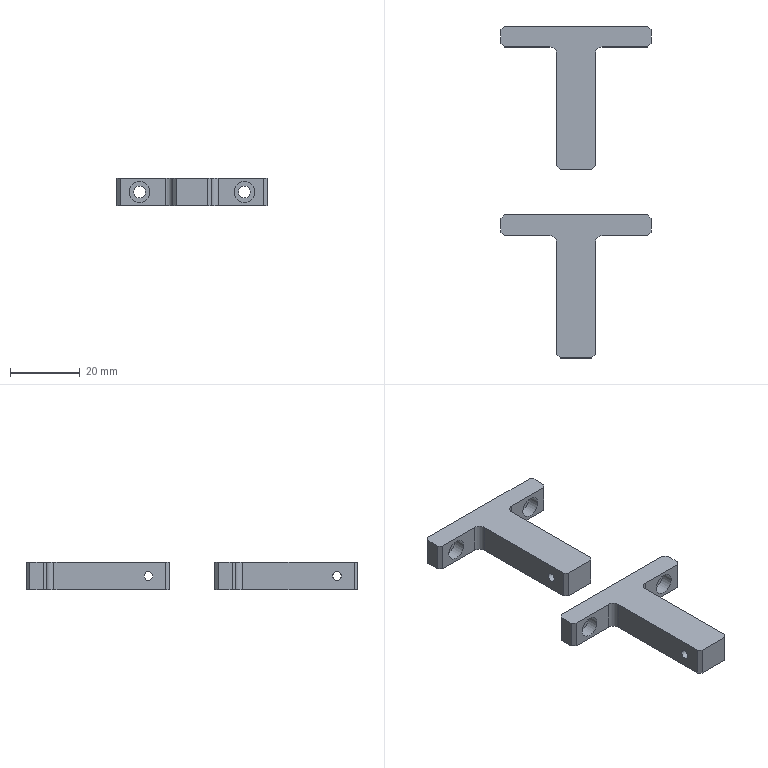Part | 2 solids | 50 faces | box 43 x 95 x 8 mm | volume 9684 mm3 | plane 36 | cylinder 14 | commonest cylinder face diameters 3.4 x4 4 x4 6 x4 2.459 x2
STEP:
#1=CARTESIAN_POINT('',(4.5,33.5,0.));
#2=VERTEX_POINT('',#1);
#3=CARTESIAN_POINT('',(-4.5,33.5,0.));
#4=VERTEX_POINT('',#3);
#5=CARTESIAN_POINT('',(21.5,33.5,0.));
#6=DIRECTION('',(-1.,0.,0.));
#7=VECTOR('',#6,1000.);
#8=LINE('',#5,#7);
#9=EDGE_CURVE('',#2,#4,#8,.T.);
#10=ORIENTED_EDGE('',*,*,#9,.T.);
#11=CARTESIAN_POINT('',(-4.5,33.5,-8.));
#12=VERTEX_POINT('',#11);
#13=CARTESIAN_POINT('',(-4.5,33.5,-8.));
#14=DIRECTION('',(0.,0.,-1.));
#15=VECTOR('',#14,1000.);
#16=LINE('',#13,#15);
#17=EDGE_CURVE('',#4,#12,#16,.T.);
#18=ORIENTED_EDGE('',*,*,#17,.T.);
#19=CARTESIAN_POINT('',(4.5,33.5,-8.));
#20=VERTEX_POINT('',#19);
#21=CARTESIAN_POINT('',(21.5,33.5,-8.));
#22=DIRECTION('',(-1.,0.,0.));
#23=VECTOR('',#22,1000.);
#24=LINE('',#21,#23);
#25=EDGE_CURVE('',#20,#12,#24,.T.);
#26=ORIENTED_EDGE('',*,*,#25,.F.);
#27=CARTESIAN_POINT('',(4.5,33.5,-8.));
#28=DIRECTION('',(0.,0.,1.));
#29=VECTOR('',#28,1000.);
#30=LINE('',#27,#29);
#31=EDGE_CURVE('',#20,#2,#30,.T.);
#32=ORIENTED_EDGE('',*,*,#31,.T.);
#33=EDGE_LOOP('',(#10,#18,#26,#32));
#34=FACE_BOUND('',#33,.T.);
#35=CARTESIAN_POINT('',(21.5,33.5,-8.));
#36=DIRECTION('',(0.,1.,0.));
#37=DIRECTION('',(0.,0.,-1.));
#38=AXIS2_PLACEMENT_3D('',#35,#36,#37);
#39=PLANE('',#38);
#40=ADVANCED_FACE('',(#34),#39,.F.);
#41=ORIENTED_EDGE('',*,*,#25,.T.);
#42=CARTESIAN_POINT('',(-5.5,34.5,-8.));
#43=VERTEX_POINT('',#42);
#44=CARTESIAN_POINT('',(-12.5,41.5,-8.));
#45=DIRECTION('',(-0.7071,0.7071,0.));
#46=VECTOR('',#45,1000.);
#47=LINE('',#44,#46);
#48=EDGE_CURVE('',#12,#43,#47,.T.);
#49=ORIENTED_EDGE('',*,*,#48,.T.);
#50=CARTESIAN_POINT('',(-5.5,66.5,-8.));
#51=VERTEX_POINT('',#50);
#52=CARTESIAN_POINT('',(-5.5,54.,-8.));
#53=DIRECTION('',(0.,1.,0.));
#54=VECTOR('',#53,1000.);
#55=LINE('',#52,#54);
#56=EDGE_CURVE('',#43,#51,#55,.T.);
#57=ORIENTED_EDGE('',*,*,#56,.T.);
#58=CARTESIAN_POINT('',(-7.5,68.5,-8.));
#59=VERTEX_POINT('',#58);
#60=CARTESIAN_POINT('',(-7.5,66.5,-8.));
#61=DIRECTION('',(0.,0.,1.));
#62=DIRECTION('',(-1.,0.,0.));
#63=AXIS2_PLACEMENT_3D('',#60,#61,#62);
#64=CIRCLE('',#63,2.);
#65=EDGE_CURVE('',#51,#59,#64,.T.);
#66=ORIENTED_EDGE('',*,*,#65,.T.);
#67=CARTESIAN_POINT('',(-20.5,68.5,-8.));
#68=VERTEX_POINT('',#67);
#69=CARTESIAN_POINT('',(0.,68.5,-8.));
#70=DIRECTION('',(-1.,0.,0.));
#71=VECTOR('',#70,1000.);
#72=LINE('',#69,#71);
#73=EDGE_CURVE('',#59,#68,#72,.T.);
#74=ORIENTED_EDGE('',*,*,#73,.T.);
#75=CARTESIAN_POINT('',(-21.5,69.5,-8.));
#76=VERTEX_POINT('',#75);
#77=CARTESIAN_POINT('',(-3.,51.,-8.));
#78=DIRECTION('',(-0.7071,0.7071,0.));
#79=VECTOR('',#78,1000.);
#80=LINE('',#77,#79);
#81=EDGE_CURVE('',#68,#76,#80,.T.);
#82=ORIENTED_EDGE('',*,*,#81,.T.);
#83=CARTESIAN_POINT('',(-21.5,73.5,-8.));
#84=VERTEX_POINT('',#83);
#85=CARTESIAN_POINT('',(-21.5,33.5,-8.));
#86=DIRECTION('',(0.,1.,0.));
#87=VECTOR('',#86,1000.);
#88=LINE('',#85,#87);
#89=EDGE_CURVE('',#76,#84,#88,.T.);
#90=ORIENTED_EDGE('',*,*,#89,.T.);
#91=CARTESIAN_POINT('',(-20.5,74.5,-8.));
#92=VERTEX_POINT('',#91);
#93=CARTESIAN_POINT('',(-20.5,74.5,-8.));
#94=DIRECTION('',(0.7071,0.7071,0.));
#95=VECTOR('',#94,1000.);
#96=LINE('',#93,#95);
#97=EDGE_CURVE('',#84,#92,#96,.T.);
#98=ORIENTED_EDGE('',*,*,#97,.T.);
#99=CARTESIAN_POINT('',(20.5,74.5,-8.));
#100=VERTEX_POINT('',#99);
#101=CARTESIAN_POINT('',(-21.5,74.5,-8.));
#102=DIRECTION('',(1.,0.,0.));
#103=VECTOR('',#102,1000.);
#104=LINE('',#101,#103);
#105=EDGE_CURVE('',#92,#100,#104,.T.);
#106=ORIENTED_EDGE('',*,*,#105,.T.);
#107=CARTESIAN_POINT('',(21.5,73.5,-8.));
#108=VERTEX_POINT('',#107);
#109=CARTESIAN_POINT('',(20.5,74.5,-8.));
#110=DIRECTION('',(0.7071,-0.7071,0.));
#111=VECTOR('',#110,1000.);
#112=LINE('',#109,#111);
#113=EDGE_CURVE('',#100,#108,#112,.T.);
#114=ORIENTED_EDGE('',*,*,#113,.T.);
#115=CARTESIAN_POINT('',(21.5,69.5,-8.));
#116=VERTEX_POINT('',#115);
#117=CARTESIAN_POINT('',(21.5,74.5,-8.));
#118=DIRECTION('',(0.,-1.,0.));
#119=VECTOR('',#118,1000.);
#120=LINE('',#117,#119);
#121=EDGE_CURVE('',#108,#116,#120,.T.);
#122=ORIENTED_EDGE('',*,*,#121,.T.);
#123=CARTESIAN_POINT('',(20.5,68.5,-8.));
#124=VERTEX_POINT('',#123);
#125=CARTESIAN_POINT('',(3.,51.,-8.));
#126=DIRECTION('',(-0.7071,-0.7071,0.));
#127=VECTOR('',#126,1000.);
#128=LINE('',#125,#127);
#129=EDGE_CURVE('',#116,#124,#128,.T.);
#130=ORIENTED_EDGE('',*,*,#129,.T.);
#131=CARTESIAN_POINT('',(7.5,68.5,-8.));
#132=VERTEX_POINT('',#131);
#133=CARTESIAN_POINT('',(0.,68.5,-8.));
#134=DIRECTION('',(1.,0.,0.));
#135=VECTOR('',#134,1000.);
#136=LINE('',#133,#135);
#137=EDGE_CURVE('',#132,#124,#136,.T.);
#138=ORIENTED_EDGE('',*,*,#137,.F.);
#139=CARTESIAN_POINT('',(5.5,66.5,-8.));
#140=VERTEX_POINT('',#139);
#141=CARTESIAN_POINT('',(7.5,66.5,-8.));
#142=DIRECTION('',(0.,0.,1.));
#143=DIRECTION('',(-1.,0.,0.));
#144=AXIS2_PLACEMENT_3D('',#141,#142,#143);
#145=CIRCLE('',#144,2.);
#146=EDGE_CURVE('',#132,#140,#145,.T.);
#147=ORIENTED_EDGE('',*,*,#146,.T.);
#148=CARTESIAN_POINT('',(5.5,34.5,-8.));
#149=VERTEX_POINT('',#148);
#150=CARTESIAN_POINT('',(5.5,54.,-8.));
#151=DIRECTION('',(0.,1.,0.));
#152=VECTOR('',#151,1000.);
#153=LINE('',#150,#152);
#154=EDGE_CURVE('',#149,#140,#153,.T.);
#155=ORIENTED_EDGE('',*,*,#154,.F.);
#156=CARTESIAN_POINT('',(12.5,41.5,-8.));
#157=DIRECTION('',(-0.7071,-0.7071,0.));
#158=VECTOR('',#157,1000.);
#159=LINE('',#156,#158);
#160=EDGE_CURVE('',#149,#20,#159,.T.);
#161=ORIENTED_EDGE('',*,*,#160,.T.);
#162=EDGE_LOOP('',(#41,#49,#57,#66,#74,#82,#90,#98,#106,#114,#122,#130,#138,#147,#155,#161));
#163=FACE_BOUND('',#162,.T.);
#164=CARTESIAN_POINT('',(0.,54.,-8.));
#165=DIRECTION('',(0.,0.,-1.));
#166=DIRECTION('',(1.,0.,0.));
#167=AXIS2_PLACEMENT_3D('',#164,#165,#166);
#168=PLANE('',#167);
#169=ADVANCED_FACE('',(#163),#168,.T.);
#170=ORIENTED_EDGE('',*,*,#121,.F.);
#171=CARTESIAN_POINT('',(21.5,73.5,0.));
#172=VERTEX_POINT('',#171);
#173=CARTESIAN_POINT('',(21.5,73.5,-8.));
#174=DIRECTION('',(0.,0.,1.));
#175=VECTOR('',#174,1000.);
#176=LINE('',#173,#175);
#177=EDGE_CURVE('',#108,#172,#176,.T.);
#178=ORIENTED_EDGE('',*,*,#177,.T.);
#179=CARTESIAN_POINT('',(21.5,69.5,0.));
#180=VERTEX_POINT('',#179);
#181=CARTESIAN_POINT('',(21.5,74.5,0.));
#182=DIRECTION('',(0.,-1.,0.));
#183=VECTOR('',#182,1000.);
#184=LINE('',#181,#183);
#185=EDGE_CURVE('',#172,#180,#184,.T.);
#186=ORIENTED_EDGE('',*,*,#185,.T.);
#187=CARTESIAN_POINT('',(21.5,69.5,-8.));
#188=DIRECTION('',(0.,0.,-1.));
#189=VECTOR('',#188,1000.);
#190=LINE('',#187,#189);
#191=EDGE_CURVE('',#180,#116,#190,.T.);
#192=ORIENTED_EDGE('',*,*,#191,.T.);
#193=EDGE_LOOP('',(#170,#178,#186,#192));
#194=FACE_BOUND('',#193,.T.);
#195=CARTESIAN_POINT('',(21.5,74.5,-8.));
#196=DIRECTION('',(-1.,0.,0.));
#197=DIRECTION('',(0.,0.,-1.));
#198=AXIS2_PLACEMENT_3D('',#195,#196,#197);
#199=PLANE('',#198);
#200=ADVANCED_FACE('',(#194),#199,.F.);
#201=CARTESIAN_POINT('',(-5.5,66.5,0.));
#202=VERTEX_POINT('',#201);
#203=CARTESIAN_POINT('',(-5.5,34.5,0.));
#204=VERTEX_POINT('',#203);
#205=CARTESIAN_POINT('',(-5.5,68.5,0.));
#206=DIRECTION('',(0.,-1.,0.));
#207=VECTOR('',#206,1000.);
#208=LINE('',#205,#207);
#209=EDGE_CURVE('',#202,#204,#208,.T.);
#210=ORIENTED_EDGE('',*,*,#209,.T.);
#211=CARTESIAN_POINT('',(-5.5,34.5,0.));
#212=DIRECTION('',(0.7071,-0.7071,0.));
#213=VECTOR('',#212,1000.);
#214=LINE('',#211,#213);
#215=EDGE_CURVE('',#204,#4,#214,.T.);
#216=ORIENTED_EDGE('',*,*,#215,.T.);
#217=ORIENTED_EDGE('',*,*,#9,.F.);
#218=CARTESIAN_POINT('',(5.5,34.5,0.));
#219=VERTEX_POINT('',#218);
#220=CARTESIAN_POINT('',(4.5,33.5,0.));
#221=DIRECTION('',(0.7071,0.7071,0.));
#222=VECTOR('',#221,1000.);
#223=LINE('',#220,#222);
#224=EDGE_CURVE('',#2,#219,#223,.T.);
#225=ORIENTED_EDGE('',*,*,#224,.T.);
#226=CARTESIAN_POINT('',(5.5,66.5,0.));
#227=VERTEX_POINT('',#226);
#228=CARTESIAN_POINT('',(5.5,68.5,0.));
#229=DIRECTION('',(0.,-1.,0.));
#230=VECTOR('',#229,1000.);
#231=LINE('',#228,#230);
#232=EDGE_CURVE('',#227,#219,#231,.T.);
#233=ORIENTED_EDGE('',*,*,#232,.F.);
#234=CARTESIAN_POINT('',(7.5,68.5,0.));
#235=VERTEX_POINT('',#234);
#236=CARTESIAN_POINT('',(7.5,66.5,0.));
#237=DIRECTION('',(0.,0.,-1.));
#238=DIRECTION('',(-1.,0.,0.));
#239=AXIS2_PLACEMENT_3D('',#236,#237,#238);
#240=CIRCLE('',#239,2.);
#241=EDGE_CURVE('',#227,#235,#240,.T.);
#242=ORIENTED_EDGE('',*,*,#241,.T.);
#243=CARTESIAN_POINT('',(20.5,68.5,0.));
#244=VERTEX_POINT('',#243);
#245=CARTESIAN_POINT('',(21.5,68.5,0.));
#246=DIRECTION('',(-1.,0.,0.));
#247=VECTOR('',#246,1000.);
#248=LINE('',#245,#247);
#249=EDGE_CURVE('',#244,#235,#248,.T.);
#250=ORIENTED_EDGE('',*,*,#249,.F.);
#251=CARTESIAN_POINT('',(20.5,68.5,0.));
#252=DIRECTION('',(0.7071,0.7071,0.));
#253=VECTOR('',#252,1000.);
#254=LINE('',#251,#253);
#255=EDGE_CURVE('',#244,#180,#254,.T.);
#256=ORIENTED_EDGE('',*,*,#255,.T.);
#257=ORIENTED_EDGE('',*,*,#185,.F.);
#258=CARTESIAN_POINT('',(20.5,74.5,0.));
#259=VERTEX_POINT('',#258);
#260=CARTESIAN_POINT('',(21.5,73.5,0.));
#261=DIRECTION('',(-0.7071,0.7071,0.));
#262=VECTOR('',#261,1000.);
#263=LINE('',#260,#262);
#264=EDGE_CURVE('',#172,#259,#263,.T.);
#265=ORIENTED_EDGE('',*,*,#264,.T.);
#266=CARTESIAN_POINT('',(-20.5,74.5,0.));
#267=VERTEX_POINT('',#266);
#268=CARTESIAN_POINT('',(-21.5,74.5,0.));
#269=DIRECTION('',(1.,0.,0.));
#270=VECTOR('',#269,1000.);
#271=LINE('',#268,#270);
#272=EDGE_CURVE('',#267,#259,#271,.T.);
#273=ORIENTED_EDGE('',*,*,#272,.F.);
#274=CARTESIAN_POINT('',(-21.5,73.5,0.));
#275=VERTEX_POINT('',#274);
#276=CARTESIAN_POINT('',(-20.5,74.5,0.));
#277=DIRECTION('',(-0.7071,-0.7071,0.));
#278=VECTOR('',#277,1000.);
#279=LINE('',#276,#278);
#280=EDGE_CURVE('',#267,#275,#279,.T.);
#281=ORIENTED_EDGE('',*,*,#280,.T.);
#282=CARTESIAN_POINT('',(-21.5,69.5,0.));
#283=VERTEX_POINT('',#282);
#284=CARTESIAN_POINT('',(-21.5,33.5,0.));
#285=DIRECTION('',(0.,1.,0.));
#286=VECTOR('',#285,1000.);
#287=LINE('',#284,#286);
#288=EDGE_CURVE('',#283,#275,#287,.T.);
#289=ORIENTED_EDGE('',*,*,#288,.F.);
#290=CARTESIAN_POINT('',(-20.5,68.5,0.));
#291=VERTEX_POINT('',#290);
#292=CARTESIAN_POINT('',(-21.5,69.5,0.));
#293=DIRECTION('',(0.7071,-0.7071,0.));
#294=VECTOR('',#293,1000.);
#295=LINE('',#292,#294);
#296=EDGE_CURVE('',#283,#291,#295,.T.);
#297=ORIENTED_EDGE('',*,*,#296,.T.);
#298=CARTESIAN_POINT('',(-7.5,68.5,0.));
#299=VERTEX_POINT('',#298);
#300=CARTESIAN_POINT('',(-21.5,68.5,0.));
#301=DIRECTION('',(1.,0.,0.));
#302=VECTOR('',#301,1000.);
#303=LINE('',#300,#302);
#304=EDGE_CURVE('',#291,#299,#303,.T.);
#305=ORIENTED_EDGE('',*,*,#304,.T.);
#306=CARTESIAN_POINT('',(-7.5,66.5,0.));
#307=DIRECTION('',(0.,0.,-1.));
#308=DIRECTION('',(-1.,0.,0.));
#309=AXIS2_PLACEMENT_3D('',#306,#307,#308);
#310=CIRCLE('',#309,2.);
#311=EDGE_CURVE('',#299,#202,#310,.T.);
#312=ORIENTED_EDGE('',*,*,#311,.T.);
#313=EDGE_LOOP('',(#210,#216,#217,#225,#233,#242,#250,#256,#257,#265,#273,#281,#289,#297,#305,#312));
#314=FACE_BOUND('',#313,.T.);
#315=CARTESIAN_POINT('',(0.,54.,0.));
#316=DIRECTION('',(0.,0.,-1.));
#317=DIRECTION('',(1.,0.,0.));
#318=AXIS2_PLACEMENT_3D('',#315,#316,#317);
#319=PLANE('',#318);
#320=ADVANCED_FACE('',(#314),#319,.F.);
#321=ORIENTED_EDGE('',*,*,#89,.F.);
#322=CARTESIAN_POINT('',(-21.5,69.5,0.));
#323=DIRECTION('',(0.,0.,1.));
#324=VECTOR('',#323,1000.);
#325=LINE('',#322,#324);
#326=EDGE_CURVE('',#76,#283,#325,.T.);
#327=ORIENTED_EDGE('',*,*,#326,.T.);
#328=ORIENTED_EDGE('',*,*,#288,.T.);
#329=CARTESIAN_POINT('',(-21.5,73.5,-8.));
#330=DIRECTION('',(0.,0.,-1.));
#331=VECTOR('',#330,1000.);
#332=LINE('',#329,#331);
#333=EDGE_CURVE('',#275,#84,#332,.T.);
#334=ORIENTED_EDGE('',*,*,#333,.T.);
#335=EDGE_LOOP('',(#321,#327,#328,#334));
#336=FACE_BOUND('',#335,.T.);
#337=CARTESIAN_POINT('',(-21.5,33.5,-8.));
#338=DIRECTION('',(1.,0.,0.));
#339=DIRECTION('',(0.,0.,1.));
#340=AXIS2_PLACEMENT_3D('',#337,#338,#339);
#341=PLANE('',#340);
#342=ADVANCED_FACE('',(#336),#341,.F.);
#343=CARTESIAN_POINT('',(15.,74.5,-5.7));
#344=VERTEX_POINT('',#343);
#345=CARTESIAN_POINT('',(15.,74.5,-4.));
#346=DIRECTION('',(0.,-1.,0.));
#347=DIRECTION('',(0.,0.,-1.));
#348=AXIS2_PLACEMENT_3D('',#345,#346,#347);
#349=CIRCLE('',#348,1.7);
#350=EDGE_CURVE('',#344,#344,#349,.T.);
#351=ORIENTED_EDGE('',*,*,#350,.T.);
#352=EDGE_LOOP('',(#351));
#353=FACE_BOUND('',#352,.T.);
#354=CARTESIAN_POINT('',(-15.,74.5,-5.7));
#355=VERTEX_POINT('',#354);
#356=CARTESIAN_POINT('',(-15.,74.5,-4.));
#357=DIRECTION('',(0.,-1.,0.));
#358=DIRECTION('',(0.,0.,-1.));
#359=AXIS2_PLACEMENT_3D('',#356,#357,#358);
#360=CIRCLE('',#359,1.7);
#361=EDGE_CURVE('',#355,#355,#360,.T.);
#362=ORIENTED_EDGE('',*,*,#361,.T.);
#363=EDGE_LOOP('',(#362));
#364=FACE_BOUND('',#363,.T.);
#365=ORIENTED_EDGE('',*,*,#105,.F.);
#366=CARTESIAN_POINT('',(-20.5,74.5,-8.));
#367=DIRECTION('',(0.,0.,1.));
#368=VECTOR('',#367,1000.);
#369=LINE('',#366,#368);
#370=EDGE_CURVE('',#92,#267,#369,.T.);
#371=ORIENTED_EDGE('',*,*,#370,.T.);
#372=ORIENTED_EDGE('',*,*,#272,.T.);
#373=CARTESIAN_POINT('',(20.5,74.5,-8.));
#374=DIRECTION('',(0.,0.,-1.));
#375=VECTOR('',#374,1000.);
#376=LINE('',#373,#375);
#377=EDGE_CURVE('',#259,#100,#376,.T.);
#378=ORIENTED_EDGE('',*,*,#377,.T.);
#379=EDGE_LOOP('',(#365,#371,#372,#378));
#380=FACE_BOUND('',#379,.T.);
#381=CARTESIAN_POINT('',(-21.5,74.5,-8.));
#382=DIRECTION('',(0.,-1.,0.));
#383=DIRECTION('',(0.,0.,1.));
#384=AXIS2_PLACEMENT_3D('',#381,#382,#383);
#385=PLANE('',#384);
#386=ADVANCED_FACE('',(#353,#364,#380),#385,.F.);
#387=CARTESIAN_POINT('',(15.,68.5,-7.));
#388=VERTEX_POINT('',#387);
#389=CARTESIAN_POINT('',(15.,68.5,-4.));
#390=DIRECTION('',(0.,1.,0.));
#391=DIRECTION('',(0.,0.,-1.));
#392=AXIS2_PLACEMENT_3D('',#389,#390,#391);
#393=CIRCLE('',#392,3.);
#394=EDGE_CURVE('',#388,#388,#393,.T.);
#395=ORIENTED_EDGE('',*,*,#394,.T.);
#396=EDGE_LOOP('',(#395));
#397=FACE_BOUND('',#396,.T.);
#398=ORIENTED_EDGE('',*,*,#249,.T.);
#399=CARTESIAN_POINT('',(7.5,68.5,-8.));
#400=DIRECTION('',(0.,0.,-1.));
#401=VECTOR('',#400,1000.);
#402=LINE('',#399,#401);
#403=EDGE_CURVE('',#235,#132,#402,.T.);
#404=ORIENTED_EDGE('',*,*,#403,.T.);
#405=ORIENTED_EDGE('',*,*,#137,.T.);
#406=CARTESIAN_POINT('',(20.5,68.5,-103.5));
#407=DIRECTION('',(0.,0.,1.));
#408=VECTOR('',#407,1000.);
#409=LINE('',#406,#408);
#410=EDGE_CURVE('',#124,#244,#409,.T.);
#411=ORIENTED_EDGE('',*,*,#410,.T.);
#412=EDGE_LOOP('',(#398,#404,#405,#411));
#413=FACE_BOUND('',#412,.T.);
#414=CARTESIAN_POINT('',(21.5,68.5,-103.5));
#415=DIRECTION('',(0.,1.,0.));
#416=DIRECTION('',(0.,0.,-1.));
#417=AXIS2_PLACEMENT_3D('',#414,#415,#416);
#418=PLANE('',#417);
#419=ADVANCED_FACE('',(#397,#413),#418,.F.);
#420=CARTESIAN_POINT('',(5.5,40.73,-4.));
#421=VERTEX_POINT('',#420);
#422=CARTESIAN_POINT('',(5.5,39.5,-4.));
#423=DIRECTION('',(-1.,0.,0.));
#424=DIRECTION('',(0.,1.,0.));
#425=AXIS2_PLACEMENT_3D('',#422,#423,#424);
#426=CIRCLE('',#425,1.23);
#427=EDGE_CURVE('',#421,#421,#426,.T.);
#428=ORIENTED_EDGE('',*,*,#427,.T.);
#429=EDGE_LOOP('',(#428));
#430=FACE_BOUND('',#429,.T.);
#431=ORIENTED_EDGE('',*,*,#154,.T.);
#432=CARTESIAN_POINT('',(5.5,66.5,0.));
#433=DIRECTION('',(0.,0.,1.));
#434=VECTOR('',#433,1000.);
#435=LINE('',#432,#434);
#436=EDGE_CURVE('',#140,#227,#435,.T.);
#437=ORIENTED_EDGE('',*,*,#436,.T.);
#438=ORIENTED_EDGE('',*,*,#232,.T.);
#439=CARTESIAN_POINT('',(5.5,34.5,-103.5));
#440=DIRECTION('',(0.,0.,-1.));
#441=VECTOR('',#440,1000.);
#442=LINE('',#439,#441);
#443=EDGE_CURVE('',#219,#149,#442,.T.);
#444=ORIENTED_EDGE('',*,*,#443,.T.);
#445=EDGE_LOOP('',(#431,#437,#438,#444));
#446=FACE_BOUND('',#445,.T.);
#447=CARTESIAN_POINT('',(5.5,68.5,-103.5));
#448=DIRECTION('',(-1.,0.,0.));
#449=DIRECTION('',(0.,1.,0.));
#450=AXIS2_PLACEMENT_3D('',#447,#448,#449);
#451=PLANE('',#450);
#452=ADVANCED_FACE('',(#430,#446),#451,.F.);
#453=CARTESIAN_POINT('',(-15.,68.5,-7.));
#454=VERTEX_POINT('',#453);
#455=CARTESIAN_POINT('',(-15.,68.5,-4.));
#456=DIRECTION('',(0.,1.,0.));
#457=DIRECTION('',(0.,0.,-1.));
#458=AXIS2_PLACEMENT_3D('',#455,#456,#457);
#459=CIRCLE('',#458,3.);
#460=EDGE_CURVE('',#454,#454,#459,.T.);
#461=ORIENTED_EDGE('',*,*,#460,.T.);
#462=EDGE_LOOP('',(#461));
#463=FACE_BOUND('',#462,.T.);
#464=ORIENTED_EDGE('',*,*,#304,.F.);
#465=CARTESIAN_POINT('',(-20.5,68.5,-8.));
#466=DIRECTION('',(0.,0.,-1.));
#467=VECTOR('',#466,1000.);
#468=LINE('',#465,#467);
#469=EDGE_CURVE('',#291,#68,#468,.T.);
#470=ORIENTED_EDGE('',*,*,#469,.T.);
#471=ORIENTED_EDGE('',*,*,#73,.F.);
#472=CARTESIAN_POINT('',(-7.5,68.5,0.));
#473=DIRECTION('',(0.,0.,1.));
#474=VECTOR('',#473,1000.);
#475=LINE('',#472,#474);
#476=EDGE_CURVE('',#59,#299,#475,.T.);
#477=ORIENTED_EDGE('',*,*,#476,.T.);
#478=EDGE_LOOP('',(#464,#470,#471,#477));
#479=FACE_BOUND('',#478,.T.);
#480=CARTESIAN_POINT('',(-21.5,68.5,-103.5));
#481=DIRECTION('',(0.,-1.,0.));
#482=DIRECTION('',(-1.,0.,0.));
#483=AXIS2_PLACEMENT_3D('',#480,#481,#482);
#484=PLANE('',#483);
#485=ADVANCED_FACE('',(#463,#479),#484,.T.);
#486=CARTESIAN_POINT('',(-5.5,38.27,-4.));
#487=VERTEX_POINT('',#486);
#488=CARTESIAN_POINT('',(-5.5,39.5,-4.));
#489=DIRECTION('',(-1.,0.,0.));
#490=DIRECTION('',(0.,-1.,0.));
#491=AXIS2_PLACEMENT_3D('',#488,#489,#490);
#492=CIRCLE('',#491,1.23);
#493=EDGE_CURVE('',#487,#487,#492,.T.);
#494=ORIENTED_EDGE('',*,*,#493,.F.);
#495=EDGE_LOOP('',(#494));
#496=FACE_BOUND('',#495,.T.);
#497=ORIENTED_EDGE('',*,*,#56,.F.);
#498=CARTESIAN_POINT('',(-5.5,34.5,0.));
#499=DIRECTION('',(0.,0.,1.));
#500=VECTOR('',#499,1000.);
#501=LINE('',#498,#500);
#502=EDGE_CURVE('',#43,#204,#501,.T.);
#503=ORIENTED_EDGE('',*,*,#502,.T.);
#504=ORIENTED_EDGE('',*,*,#209,.F.);
#505=CARTESIAN_POINT('',(-5.5,66.5,-8.));
#506=DIRECTION('',(0.,0.,-1.));
#507=VECTOR('',#506,1000.);
#508=LINE('',#505,#507);
#509=EDGE_CURVE('',#202,#51,#508,.T.);
#510=ORIENTED_EDGE('',*,*,#509,.T.);
#511=EDGE_LOOP('',(#497,#503,#504,#510));
#512=FACE_BOUND('',#511,.T.);
#513=CARTESIAN_POINT('',(-5.5,68.5,-103.5));
#514=DIRECTION('',(-1.,0.,0.));
#515=DIRECTION('',(0.,1.,0.));
#516=AXIS2_PLACEMENT_3D('',#513,#514,#515);
#517=PLANE('',#516);
#518=ADVANCED_FACE('',(#496,#512),#517,.T.);
#519=ORIENTED_EDGE('',*,*,#160,.F.);
#520=ORIENTED_EDGE('',*,*,#443,.F.);
#521=ORIENTED_EDGE('',*,*,#224,.F.);
#522=ORIENTED_EDGE('',*,*,#31,.F.);
#523=EDGE_LOOP('',(#519,#520,#521,#522));
#524=FACE_BOUND('',#523,.T.);
#525=CARTESIAN_POINT('',(4.5,33.5,-8.));
#526=DIRECTION('',(-0.7071,0.7071,0.));
#527=DIRECTION('',(0.,0.,-1.));
#528=AXIS2_PLACEMENT_3D('',#525,#526,#527);
#529=PLANE('',#528);
#530=ADVANCED_FACE('',(#524),#529,.F.);
#531=ORIENTED_EDGE('',*,*,#97,.F.);
#532=ORIENTED_EDGE('',*,*,#333,.F.);
#533=ORIENTED_EDGE('',*,*,#280,.F.);
#534=ORIENTED_EDGE('',*,*,#370,.F.);
#535=EDGE_LOOP('',(#531,#532,#533,#534));
#536=FACE_BOUND('',#535,.T.);
#537=CARTESIAN_POINT('',(-20.5,74.5,-8.));
#538=DIRECTION('',(0.7071,-0.7071,0.));
#539=DIRECTION('',(0.,0.,-1.));
#540=AXIS2_PLACEMENT_3D('',#537,#538,#539);
#541=PLANE('',#540);
#542=ADVANCED_FACE('',(#536),#541,.F.);
#543=ORIENTED_EDGE('',*,*,#113,.F.);
#544=ORIENTED_EDGE('',*,*,#377,.F.);
#545=ORIENTED_EDGE('',*,*,#264,.F.);
#546=ORIENTED_EDGE('',*,*,#177,.F.);
#547=EDGE_LOOP('',(#543,#544,#545,#546));
#548=FACE_BOUND('',#547,.T.);
#549=CARTESIAN_POINT('',(21.5,73.5,-8.));
#550=DIRECTION('',(-0.7071,-0.7071,0.));
#551=DIRECTION('',(0.,0.,-1.));
#552=AXIS2_PLACEMENT_3D('',#549,#550,#551);
#553=PLANE('',#552);
#554=ADVANCED_FACE('',(#548),#553,.F.);
#555=ORIENTED_EDGE('',*,*,#129,.F.);
#556=ORIENTED_EDGE('',*,*,#191,.F.);
#557=ORIENTED_EDGE('',*,*,#255,.F.);
#558=ORIENTED_EDGE('',*,*,#410,.F.);
#559=EDGE_LOOP('',(#555,#556,#557,#558));
#560=FACE_BOUND('',#559,.T.);
#561=CARTESIAN_POINT('',(20.5,68.5,-103.5));
#562=DIRECTION('',(-0.7071,0.7071,0.));
#563=DIRECTION('',(0.,0.,-1.));
#564=AXIS2_PLACEMENT_3D('',#561,#562,#563);
#565=PLANE('',#564);
#566=ADVANCED_FACE('',(#560),#565,.F.);
#567=ORIENTED_EDGE('',*,*,#146,.F.);
#568=ORIENTED_EDGE('',*,*,#403,.F.);
#569=ORIENTED_EDGE('',*,*,#241,.F.);
#570=ORIENTED_EDGE('',*,*,#436,.F.);
#571=EDGE_LOOP('',(#567,#568,#569,#570));
#572=FACE_BOUND('',#571,.T.);
#573=CARTESIAN_POINT('',(7.5,66.5,-103.5));
#574=DIRECTION('',(0.,0.,-1.));
#575=DIRECTION('',(1.,0.,0.));
#576=AXIS2_PLACEMENT_3D('',#573,#574,#575);
#577=CYLINDRICAL_SURFACE('',#576,2.);
#578=ADVANCED_FACE('',(#572),#577,.F.);
#579=ORIENTED_EDGE('',*,*,#65,.F.);
#580=ORIENTED_EDGE('',*,*,#509,.F.);
#581=ORIENTED_EDGE('',*,*,#311,.F.);
#582=ORIENTED_EDGE('',*,*,#476,.F.);
#583=EDGE_LOOP('',(#579,#580,#581,#582));
#584=FACE_BOUND('',#583,.T.);
#585=CARTESIAN_POINT('',(-7.5,66.5,-103.5));
#586=DIRECTION('',(0.,0.,-1.));
#587=DIRECTION('',(1.,0.,0.));
#588=AXIS2_PLACEMENT_3D('',#585,#586,#587);
#589=CYLINDRICAL_SURFACE('',#588,2.);
#590=ADVANCED_FACE('',(#584),#589,.F.);
#591=CARTESIAN_POINT('',(-15.,71.9,-5.7));
#592=VERTEX_POINT('',#591);
#593=CARTESIAN_POINT('',(-15.,71.9,-4.));
#594=DIRECTION('',(0.,1.,0.));
#595=DIRECTION('',(0.,0.,-1.));
#596=AXIS2_PLACEMENT_3D('',#593,#594,#595);
#597=CIRCLE('',#596,1.7);
#598=EDGE_CURVE('',#592,#592,#597,.T.);
#599=ORIENTED_EDGE('',*,*,#598,.F.);
#600=EDGE_LOOP('',(#599));
#601=FACE_BOUND('',#600,.T.);
#602=ORIENTED_EDGE('',*,*,#361,.F.);
#603=EDGE_LOOP('',(#602));
#604=FACE_BOUND('',#603,.T.);
#605=CARTESIAN_POINT('',(-15.,71.9,-4.));
#606=DIRECTION('',(0.,1.,0.));
#607=DIRECTION('',(0.,0.,1.));
#608=AXIS2_PLACEMENT_3D('',#605,#606,#607);
#609=CYLINDRICAL_SURFACE('',#608,1.7);
#610=ADVANCED_FACE('',(#601,#604),#609,.F.);
#611=ORIENTED_EDGE('',*,*,#598,.T.);
#612=EDGE_LOOP('',(#611));
#613=FACE_BOUND('',#612,.T.);
#614=CARTESIAN_POINT('',(-15.,71.9,-7.));
#615=VERTEX_POINT('',#614);
#616=CARTESIAN_POINT('',(-15.,71.9,-4.));
#617=DIRECTION('',(0.,-1.,0.));
#618=DIRECTION('',(0.,0.,-1.));
#619=AXIS2_PLACEMENT_3D('',#616,#617,#618);
#620=CIRCLE('',#619,3.);
#621=EDGE_CURVE('',#615,#615,#620,.T.);
#622=ORIENTED_EDGE('',*,*,#621,.T.);
#623=EDGE_LOOP('',(#622));
#624=FACE_BOUND('',#623,.T.);
#625=CARTESIAN_POINT('',(-15.,71.9,-4.));
#626=DIRECTION('',(0.,1.,0.));
#627=DIRECTION('',(0.,0.,-1.));
#628=AXIS2_PLACEMENT_3D('',#625,#626,#627);
#629=PLANE('',#628);
#630=ADVANCED_FACE('',(#613,#624),#629,.F.);
#631=ORIENTED_EDGE('',*,*,#621,.F.);
#632=EDGE_LOOP('',(#631));
#633=FACE_BOUND('',#632,.T.);
#634=ORIENTED_EDGE('',*,*,#460,.F.);
#635=EDGE_LOOP('',(#634));
#636=FACE_BOUND('',#635,.T.);
#637=CARTESIAN_POINT('',(-15.,68.5,-4.));
#638=DIRECTION('',(0.,1.,0.));
#639=DIRECTION('',(0.,0.,1.));
#640=AXIS2_PLACEMENT_3D('',#637,#638,#639);
#641=CYLINDRICAL_SURFACE('',#640,3.);
#642=ADVANCED_FACE('',(#633,#636),#641,.F.);
#643=CARTESIAN_POINT('',(15.,71.9,-5.7));
#644=VERTEX_POINT('',#643);
#645=CARTESIAN_POINT('',(15.,71.9,-4.));
#646=DIRECTION('',(0.,1.,0.));
#647=DIRECTION('',(0.,0.,-1.));
#648=AXIS2_PLACEMENT_3D('',#645,#646,#647);
#649=CIRCLE('',#648,1.7);
#650=EDGE_CURVE('',#644,#644,#649,.T.);
#651=ORIENTED_EDGE('',*,*,#650,.F.);
#652=EDGE_LOOP('',(#651));
#653=FACE_BOUND('',#652,.T.);
#654=ORIENTED_EDGE('',*,*,#350,.F.);
#655=EDGE_LOOP('',(#654));
#656=FACE_BOUND('',#655,.T.);
#657=CARTESIAN_POINT('',(15.,71.9,-4.));
#658=DIRECTION('',(0.,1.,0.));
#659=DIRECTION('',(0.,0.,1.));
#660=AXIS2_PLACEMENT_3D('',#657,#658,#659);
#661=CYLINDRICAL_SURFACE('',#660,1.7);
#662=ADVANCED_FACE('',(#653,#656),#661,.F.);
#663=ORIENTED_EDGE('',*,*,#650,.T.);
#664=EDGE_LOOP('',(#663));
#665=FACE_BOUND('',#664,.T.);
#666=CARTESIAN_POINT('',(15.,71.9,-7.));
#667=VERTEX_POINT('',#666);
#668=CARTESIAN_POINT('',(15.,71.9,-4.));
#669=DIRECTION('',(0.,-1.,0.));
#670=DIRECTION('',(0.,0.,-1.));
#671=AXIS2_PLACEMENT_3D('',#668,#669,#670);
#672=CIRCLE('',#671,3.);
#673=EDGE_CURVE('',#667,#667,#672,.T.);
#674=ORIENTED_EDGE('',*,*,#673,.T.);
#675=EDGE_LOOP('',(#674));
#676=FACE_BOUND('',#675,.T.);
#677=CARTESIAN_POINT('',(15.,71.9,-4.));
#678=DIRECTION('',(0.,1.,0.));
#679=DIRECTION('',(0.,0.,-1.));
#680=AXIS2_PLACEMENT_3D('',#677,#678,#679);
#681=PLANE('',#680);
#682=ADVANCED_FACE('',(#665,#676),#681,.F.);
#683=ORIENTED_EDGE('',*,*,#673,.F.);
#684=EDGE_LOOP('',(#683));
#685=FACE_BOUND('',#684,.T.);
#686=ORIENTED_EDGE('',*,*,#394,.F.);
#687=EDGE_LOOP('',(#686));
#688=FACE_BOUND('',#687,.T.);
#689=CARTESIAN_POINT('',(15.,68.5,-4.));
#690=DIRECTION('',(0.,1.,0.));
#691=DIRECTION('',(0.,0.,1.));
#692=AXIS2_PLACEMENT_3D('',#689,#690,#691);
#693=CYLINDRICAL_SURFACE('',#692,3.);
#694=ADVANCED_FACE('',(#685,#688),#693,.F.);
#695=ORIENTED_EDGE('',*,*,#493,.T.);
#696=EDGE_LOOP('',(#695));
#697=FACE_BOUND('',#696,.T.);
#698=ORIENTED_EDGE('',*,*,#427,.F.);
#699=EDGE_LOOP('',(#698));
#700=FACE_BOUND('',#699,.T.);
#701=CARTESIAN_POINT('',(5.5,39.5,-4.));
#702=DIRECTION('',(-1.,0.,0.));
#703=DIRECTION('',(0.,-1.,0.));
#704=AXIS2_PLACEMENT_3D('',#701,#702,#703);
#705=CYLINDRICAL_SURFACE('',#704,1.23);
#706=ADVANCED_FACE('',(#697,#700),#705,.F.);
#707=ORIENTED_EDGE('',*,*,#81,.F.);
#708=ORIENTED_EDGE('',*,*,#469,.F.);
#709=ORIENTED_EDGE('',*,*,#296,.F.);
#710=ORIENTED_EDGE('',*,*,#326,.F.);
#711=EDGE_LOOP('',(#707,#708,#709,#710));
#712=FACE_BOUND('',#711,.T.);
#713=CARTESIAN_POINT('',(-21.5,69.5,-8.));
#714=DIRECTION('',(-0.7071,-0.7071,0.));
#715=DIRECTION('',(0.,0.,1.));
#716=AXIS2_PLACEMENT_3D('',#713,#714,#715);
#717=PLANE('',#716);
#718=ADVANCED_FACE('',(#712),#717,.T.);
#719=ORIENTED_EDGE('',*,*,#48,.F.);
#720=ORIENTED_EDGE('',*,*,#17,.F.);
#721=ORIENTED_EDGE('',*,*,#215,.F.);
#722=ORIENTED_EDGE('',*,*,#502,.F.);
#723=EDGE_LOOP('',(#719,#720,#721,#722));
#724=FACE_BOUND('',#723,.T.);
#725=CARTESIAN_POINT('',(-5.5,34.5,-103.5));
#726=DIRECTION('',(-0.7071,-0.7071,0.));
#727=DIRECTION('',(0.,0.,1.));
#728=AXIS2_PLACEMENT_3D('',#725,#726,#727);
#729=PLANE('',#728);
#730=ADVANCED_FACE('',(#724),#729,.T.);
#731=CLOSED_SHELL('',(#40,#169,#200,#320,#342,#386,#419,#452,#485,#518,#530,#542,#554,#566,#578,#590,#610,#630,#642,#662,#682,#694,#706,#718,#730));
#732=MANIFOLD_SOLID_BREP('',#731);
#733=CARTESIAN_POINT('',(4.5,-20.5,0.));
#734=VERTEX_POINT('',#733);
#735=CARTESIAN_POINT('',(-4.5,-20.5,0.));
#736=VERTEX_POINT('',#735);
#737=CARTESIAN_POINT('',(21.5,-20.5,0.));
#738=DIRECTION('',(-1.,0.,0.));
#739=VECTOR('',#738,1000.);
#740=LINE('',#737,#739);
#741=EDGE_CURVE('',#734,#736,#740,.T.);
#742=ORIENTED_EDGE('',*,*,#741,.T.);
#743=CARTESIAN_POINT('',(-4.5,-20.5,-8.));
#744=VERTEX_POINT('',#743);
#745=CARTESIAN_POINT('',(-4.5,-20.5,-8.));
#746=DIRECTION('',(0.,0.,-1.));
#747=VECTOR('',#746,1000.);
#748=LINE('',#745,#747);
#749=EDGE_CURVE('',#736,#744,#748,.T.);
#750=ORIENTED_EDGE('',*,*,#749,.T.);
#751=CARTESIAN_POINT('',(4.5,-20.5,-8.));
#752=VERTEX_POINT('',#751);
#753=CARTESIAN_POINT('',(21.5,-20.5,-8.));
#754=DIRECTION('',(-1.,0.,0.));
#755=VECTOR('',#754,1000.);
#756=LINE('',#753,#755);
#757=EDGE_CURVE('',#752,#744,#756,.T.);
#758=ORIENTED_EDGE('',*,*,#757,.F.);
#759=CARTESIAN_POINT('',(4.5,-20.5,-8.));
#760=DIRECTION('',(0.,0.,1.));
#761=VECTOR('',#760,1000.);
#762=LINE('',#759,#761);
#763=EDGE_CURVE('',#752,#734,#762,.T.);
#764=ORIENTED_EDGE('',*,*,#763,.T.);
#765=EDGE_LOOP('',(#742,#750,#758,#764));
#766=FACE_BOUND('',#765,.T.);
#767=CARTESIAN_POINT('',(21.5,-20.5,-8.));
#768=DIRECTION('',(0.,1.,0.));
#769=DIRECTION('',(0.,0.,-1.));
#770=AXIS2_PLACEMENT_3D('',#767,#768,#769);
#771=PLANE('',#770);
#772=ADVANCED_FACE('',(#766),#771,.F.);
#773=ORIENTED_EDGE('',*,*,#757,.T.);
#774=CARTESIAN_POINT('',(-5.5,-19.5,-8.));
#775=VERTEX_POINT('',#774);
#776=CARTESIAN_POINT('',(-12.5,-12.5,-8.));
#777=DIRECTION('',(-0.7071,0.7071,0.));
#778=VECTOR('',#777,1000.);
#779=LINE('',#776,#778);
#780=EDGE_CURVE('',#744,#775,#779,.T.);
#781=ORIENTED_EDGE('',*,*,#780,.T.);
#782=CARTESIAN_POINT('',(-5.5,12.5,-8.));
#783=VERTEX_POINT('',#782);
#784=CARTESIAN_POINT('',(-5.5,0.,-8.));
#785=DIRECTION('',(0.,1.,0.));
#786=VECTOR('',#785,1000.);
#787=LINE('',#784,#786);
#788=EDGE_CURVE('',#775,#783,#787,.T.);
#789=ORIENTED_EDGE('',*,*,#788,.T.);
#790=CARTESIAN_POINT('',(-7.5,14.5,-8.));
#791=VERTEX_POINT('',#790);
#792=CARTESIAN_POINT('',(-7.5,12.5,-8.));
#793=DIRECTION('',(0.,0.,1.));
#794=DIRECTION('',(-1.,0.,0.));
#795=AXIS2_PLACEMENT_3D('',#792,#793,#794);
#796=CIRCLE('',#795,2.);
#797=EDGE_CURVE('',#783,#791,#796,.T.);
#798=ORIENTED_EDGE('',*,*,#797,.T.);
#799=CARTESIAN_POINT('',(-20.5,14.5,-8.));
#800=VERTEX_POINT('',#799);
#801=CARTESIAN_POINT('',(0.,14.5,-8.));
#802=DIRECTION('',(-1.,0.,0.));
#803=VECTOR('',#802,1000.);
#804=LINE('',#801,#803);
#805=EDGE_CURVE('',#791,#800,#804,.T.);
#806=ORIENTED_EDGE('',*,*,#805,.T.);
#807=CARTESIAN_POINT('',(-21.5,15.5,-8.));
#808=VERTEX_POINT('',#807);
#809=CARTESIAN_POINT('',(-3.,-3.,-8.));
#810=DIRECTION('',(-0.7071,0.7071,0.));
#811=VECTOR('',#810,1000.);
#812=LINE('',#809,#811);
#813=EDGE_CURVE('',#800,#808,#812,.T.);
#814=ORIENTED_EDGE('',*,*,#813,.T.);
#815=CARTESIAN_POINT('',(-21.5,19.5,-8.));
#816=VERTEX_POINT('',#815);
#817=CARTESIAN_POINT('',(-21.5,-20.5,-8.));
#818=DIRECTION('',(0.,1.,0.));
#819=VECTOR('',#818,1000.);
#820=LINE('',#817,#819);
#821=EDGE_CURVE('',#808,#816,#820,.T.);
#822=ORIENTED_EDGE('',*,*,#821,.T.);
#823=CARTESIAN_POINT('',(-20.5,20.5,-8.));
#824=VERTEX_POINT('',#823);
#825=CARTESIAN_POINT('',(-20.5,20.5,-8.));
#826=DIRECTION('',(0.7071,0.7071,0.));
#827=VECTOR('',#826,1000.);
#828=LINE('',#825,#827);
#829=EDGE_CURVE('',#816,#824,#828,.T.);
#830=ORIENTED_EDGE('',*,*,#829,.T.);
#831=CARTESIAN_POINT('',(20.5,20.5,-8.));
#832=VERTEX_POINT('',#831);
#833=CARTESIAN_POINT('',(-21.5,20.5,-8.));
#834=DIRECTION('',(1.,0.,0.));
#835=VECTOR('',#834,1000.);
#836=LINE('',#833,#835);
#837=EDGE_CURVE('',#824,#832,#836,.T.);
#838=ORIENTED_EDGE('',*,*,#837,.T.);
#839=CARTESIAN_POINT('',(21.5,19.5,-8.));
#840=VERTEX_POINT('',#839);
#841=CARTESIAN_POINT('',(20.5,20.5,-8.));
#842=DIRECTION('',(0.7071,-0.7071,0.));
#843=VECTOR('',#842,1000.);
#844=LINE('',#841,#843);
#845=EDGE_CURVE('',#832,#840,#844,.T.);
#846=ORIENTED_EDGE('',*,*,#845,.T.);
#847=CARTESIAN_POINT('',(21.5,15.5,-8.));
#848=VERTEX_POINT('',#847);
#849=CARTESIAN_POINT('',(21.5,20.5,-8.));
#850=DIRECTION('',(0.,-1.,0.));
#851=VECTOR('',#850,1000.);
#852=LINE('',#849,#851);
#853=EDGE_CURVE('',#840,#848,#852,.T.);
#854=ORIENTED_EDGE('',*,*,#853,.T.);
#855=CARTESIAN_POINT('',(20.5,14.5,-8.));
#856=VERTEX_POINT('',#855);
#857=CARTESIAN_POINT('',(3.,-3.,-8.));
#858=DIRECTION('',(-0.7071,-0.7071,0.));
#859=VECTOR('',#858,1000.);
#860=LINE('',#857,#859);
#861=EDGE_CURVE('',#848,#856,#860,.T.);
#862=ORIENTED_EDGE('',*,*,#861,.T.);
#863=CARTESIAN_POINT('',(7.5,14.5,-8.));
#864=VERTEX_POINT('',#863);
#865=CARTESIAN_POINT('',(0.,14.5,-8.));
#866=DIRECTION('',(1.,0.,0.));
#867=VECTOR('',#866,1000.);
#868=LINE('',#865,#867);
#869=EDGE_CURVE('',#864,#856,#868,.T.);
#870=ORIENTED_EDGE('',*,*,#869,.F.);
#871=CARTESIAN_POINT('',(5.5,12.5,-8.));
#872=VERTEX_POINT('',#871);
#873=CARTESIAN_POINT('',(7.5,12.5,-8.));
#874=DIRECTION('',(0.,0.,1.));
#875=DIRECTION('',(-1.,0.,0.));
#876=AXIS2_PLACEMENT_3D('',#873,#874,#875);
#877=CIRCLE('',#876,2.);
#878=EDGE_CURVE('',#864,#872,#877,.T.);
#879=ORIENTED_EDGE('',*,*,#878,.T.);
#880=CARTESIAN_POINT('',(5.5,-19.5,-8.));
#881=VERTEX_POINT('',#880);
#882=CARTESIAN_POINT('',(5.5,0.,-8.));
#883=DIRECTION('',(0.,1.,0.));
#884=VECTOR('',#883,1000.);
#885=LINE('',#882,#884);
#886=EDGE_CURVE('',#881,#872,#885,.T.);
#887=ORIENTED_EDGE('',*,*,#886,.F.);
#888=CARTESIAN_POINT('',(12.5,-12.5,-8.));
#889=DIRECTION('',(-0.7071,-0.7071,0.));
#890=VECTOR('',#889,1000.);
#891=LINE('',#888,#890);
#892=EDGE_CURVE('',#881,#752,#891,.T.);
#893=ORIENTED_EDGE('',*,*,#892,.T.);
#894=EDGE_LOOP('',(#773,#781,#789,#798,#806,#814,#822,#830,#838,#846,#854,#862,#870,#879,#887,#893));
#895=FACE_BOUND('',#894,.T.);
#896=CARTESIAN_POINT('',(0.,0.,-8.));
#897=DIRECTION('',(0.,0.,-1.));
#898=DIRECTION('',(1.,0.,0.));
#899=AXIS2_PLACEMENT_3D('',#896,#897,#898);
#900=PLANE('',#899);
#901=ADVANCED_FACE('',(#895),#900,.T.);
#902=ORIENTED_EDGE('',*,*,#853,.F.);
#903=CARTESIAN_POINT('',(21.5,19.5,0.));
#904=VERTEX_POINT('',#903);
#905=CARTESIAN_POINT('',(21.5,19.5,-8.));
#906=DIRECTION('',(0.,0.,1.));
#907=VECTOR('',#906,1000.);
#908=LINE('',#905,#907);
#909=EDGE_CURVE('',#840,#904,#908,.T.);
#910=ORIENTED_EDGE('',*,*,#909,.T.);
#911=CARTESIAN_POINT('',(21.5,15.5,0.));
#912=VERTEX_POINT('',#911);
#913=CARTESIAN_POINT('',(21.5,20.5,0.));
#914=DIRECTION('',(0.,-1.,0.));
#915=VECTOR('',#914,1000.);
#916=LINE('',#913,#915);
#917=EDGE_CURVE('',#904,#912,#916,.T.);
#918=ORIENTED_EDGE('',*,*,#917,.T.);
#919=CARTESIAN_POINT('',(21.5,15.5,-8.));
#920=DIRECTION('',(0.,0.,-1.));
#921=VECTOR('',#920,1000.);
#922=LINE('',#919,#921);
#923=EDGE_CURVE('',#912,#848,#922,.T.);
#924=ORIENTED_EDGE('',*,*,#923,.T.);
#925=EDGE_LOOP('',(#902,#910,#918,#924));
#926=FACE_BOUND('',#925,.T.);
#927=CARTESIAN_POINT('',(21.5,20.5,-8.));
#928=DIRECTION('',(-1.,0.,0.));
#929=DIRECTION('',(0.,0.,-1.));
#930=AXIS2_PLACEMENT_3D('',#927,#928,#929);
#931=PLANE('',#930);
#932=ADVANCED_FACE('',(#926),#931,.F.);
#933=CARTESIAN_POINT('',(-5.5,12.5,0.));
#934=VERTEX_POINT('',#933);
#935=CARTESIAN_POINT('',(-5.5,-19.5,0.));
#936=VERTEX_POINT('',#935);
#937=CARTESIAN_POINT('',(-5.5,14.5,0.));
#938=DIRECTION('',(0.,-1.,0.));
#939=VECTOR('',#938,1000.);
#940=LINE('',#937,#939);
#941=EDGE_CURVE('',#934,#936,#940,.T.);
#942=ORIENTED_EDGE('',*,*,#941,.T.);
#943=CARTESIAN_POINT('',(-5.5,-19.5,0.));
#944=DIRECTION('',(0.7071,-0.7071,0.));
#945=VECTOR('',#944,1000.);
#946=LINE('',#943,#945);
#947=EDGE_CURVE('',#936,#736,#946,.T.);
#948=ORIENTED_EDGE('',*,*,#947,.T.);
#949=ORIENTED_EDGE('',*,*,#741,.F.);
#950=CARTESIAN_POINT('',(5.5,-19.5,0.));
#951=VERTEX_POINT('',#950);
#952=CARTESIAN_POINT('',(4.5,-20.5,0.));
#953=DIRECTION('',(0.7071,0.7071,0.));
#954=VECTOR('',#953,1000.);
#955=LINE('',#952,#954);
#956=EDGE_CURVE('',#734,#951,#955,.T.);
#957=ORIENTED_EDGE('',*,*,#956,.T.);
#958=CARTESIAN_POINT('',(5.5,12.5,0.));
#959=VERTEX_POINT('',#958);
#960=CARTESIAN_POINT('',(5.5,14.5,0.));
#961=DIRECTION('',(0.,-1.,0.));
#962=VECTOR('',#961,1000.);
#963=LINE('',#960,#962);
#964=EDGE_CURVE('',#959,#951,#963,.T.);
#965=ORIENTED_EDGE('',*,*,#964,.F.);
#966=CARTESIAN_POINT('',(7.5,14.5,0.));
#967=VERTEX_POINT('',#966);
#968=CARTESIAN_POINT('',(7.5,12.5,0.));
#969=DIRECTION('',(0.,0.,-1.));
#970=DIRECTION('',(-1.,0.,0.));
#971=AXIS2_PLACEMENT_3D('',#968,#969,#970);
#972=CIRCLE('',#971,2.);
#973=EDGE_CURVE('',#959,#967,#972,.T.);
#974=ORIENTED_EDGE('',*,*,#973,.T.);
#975=CARTESIAN_POINT('',(20.5,14.5,0.));
#976=VERTEX_POINT('',#975);
#977=CARTESIAN_POINT('',(21.5,14.5,0.));
#978=DIRECTION('',(-1.,0.,0.));
#979=VECTOR('',#978,1000.);
#980=LINE('',#977,#979);
#981=EDGE_CURVE('',#976,#967,#980,.T.);
#982=ORIENTED_EDGE('',*,*,#981,.F.);
#983=CARTESIAN_POINT('',(20.5,14.5,0.));
#984=DIRECTION('',(0.7071,0.7071,0.));
#985=VECTOR('',#984,1000.);
#986=LINE('',#983,#985);
#987=EDGE_CURVE('',#976,#912,#986,.T.);
#988=ORIENTED_EDGE('',*,*,#987,.T.);
#989=ORIENTED_EDGE('',*,*,#917,.F.);
#990=CARTESIAN_POINT('',(20.5,20.5,0.));
#991=VERTEX_POINT('',#990);
#992=CARTESIAN_POINT('',(21.5,19.5,0.));
#993=DIRECTION('',(-0.7071,0.7071,0.));
#994=VECTOR('',#993,1000.);
#995=LINE('',#992,#994);
#996=EDGE_CURVE('',#904,#991,#995,.T.);
#997=ORIENTED_EDGE('',*,*,#996,.T.);
#998=CARTESIAN_POINT('',(-20.5,20.5,0.));
#999=VERTEX_POINT('',#998);
#1000=CARTESIAN_POINT('',(-21.5,20.5,0.));
#1001=DIRECTION('',(1.,0.,0.));
#1002=VECTOR('',#1001,1000.);
#1003=LINE('',#1000,#1002);
#1004=EDGE_CURVE('',#999,#991,#1003,.T.);
#1005=ORIENTED_EDGE('',*,*,#1004,.F.);
#1006=CARTESIAN_POINT('',(-21.5,19.5,0.));
#1007=VERTEX_POINT('',#1006);
#1008=CARTESIAN_POINT('',(-20.5,20.5,0.));
#1009=DIRECTION('',(-0.7071,-0.7071,0.));
#1010=VECTOR('',#1009,1000.);
#1011=LINE('',#1008,#1010);
#1012=EDGE_CURVE('',#999,#1007,#1011,.T.);
#1013=ORIENTED_EDGE('',*,*,#1012,.T.);
#1014=CARTESIAN_POINT('',(-21.5,15.5,0.));
#1015=VERTEX_POINT('',#1014);
#1016=CARTESIAN_POINT('',(-21.5,-20.5,0.));
#1017=DIRECTION('',(0.,1.,0.));
#1018=VECTOR('',#1017,1000.);
#1019=LINE('',#1016,#1018);
#1020=EDGE_CURVE('',#1015,#1007,#1019,.T.);
#1021=ORIENTED_EDGE('',*,*,#1020,.F.);
#1022=CARTESIAN_POINT('',(-20.5,14.5,0.));
#1023=VERTEX_POINT('',#1022);
#1024=CARTESIAN_POINT('',(-21.5,15.5,0.));
#1025=DIRECTION('',(0.7071,-0.7071,0.));
#1026=VECTOR('',#1025,1000.);
#1027=LINE('',#1024,#1026);
#1028=EDGE_CURVE('',#1015,#1023,#1027,.T.);
#1029=ORIENTED_EDGE('',*,*,#1028,.T.);
#1030=CARTESIAN_POINT('',(-7.5,14.5,0.));
#1031=VERTEX_POINT('',#1030);
#1032=CARTESIAN_POINT('',(-21.5,14.5,0.));
#1033=DIRECTION('',(1.,0.,0.));
#1034=VECTOR('',#1033,1000.);
#1035=LINE('',#1032,#1034);
#1036=EDGE_CURVE('',#1023,#1031,#1035,.T.);
#1037=ORIENTED_EDGE('',*,*,#1036,.T.);
#1038=CARTESIAN_POINT('',(-7.5,12.5,0.));
#1039=DIRECTION('',(0.,0.,-1.));
#1040=DIRECTION('',(-1.,0.,0.));
#1041=AXIS2_PLACEMENT_3D('',#1038,#1039,#1040);
#1042=CIRCLE('',#1041,2.);
#1043=EDGE_CURVE('',#1031,#934,#1042,.T.);
#1044=ORIENTED_EDGE('',*,*,#1043,.T.);
#1045=EDGE_LOOP('',(#942,#948,#949,#957,#965,#974,#982,#988,#989,#997,#1005,#1013,#1021,#1029,#1037,#1044));
#1046=FACE_BOUND('',#1045,.T.);
#1047=CARTESIAN_POINT('',(0.,0.,0.));
#1048=DIRECTION('',(0.,0.,-1.));
#1049=DIRECTION('',(1.,0.,0.));
#1050=AXIS2_PLACEMENT_3D('',#1047,#1048,#1049);
#1051=PLANE('',#1050);
#1052=ADVANCED_FACE('',(#1046),#1051,.F.);
#1053=ORIENTED_EDGE('',*,*,#821,.F.);
#1054=CARTESIAN_POINT('',(-21.5,15.5,0.));
#1055=DIRECTION('',(0.,0.,1.));
#1056=VECTOR('',#1055,1000.);
#1057=LINE('',#1054,#1056);
#1058=EDGE_CURVE('',#808,#1015,#1057,.T.);
#1059=ORIENTED_EDGE('',*,*,#1058,.T.);
#1060=ORIENTED_EDGE('',*,*,#1020,.T.);
#1061=CARTESIAN_POINT('',(-21.5,19.5,-8.));
#1062=DIRECTION('',(0.,0.,-1.));
#1063=VECTOR('',#1062,1000.);
#1064=LINE('',#1061,#1063);
#1065=EDGE_CURVE('',#1007,#816,#1064,.T.);
#1066=ORIENTED_EDGE('',*,*,#1065,.T.);
#1067=EDGE_LOOP('',(#1053,#1059,#1060,#1066));
#1068=FACE_BOUND('',#1067,.T.);
#1069=CARTESIAN_POINT('',(-21.5,-20.5,-8.));
#1070=DIRECTION('',(1.,0.,0.));
#1071=DIRECTION('',(0.,0.,1.));
#1072=AXIS2_PLACEMENT_3D('',#1069,#1070,#1071);
#1073=PLANE('',#1072);
#1074=ADVANCED_FACE('',(#1068),#1073,.F.);
#1075=CARTESIAN_POINT('',(15.,20.5,-5.7));
#1076=VERTEX_POINT('',#1075);
#1077=CARTESIAN_POINT('',(15.,20.5,-4.));
#1078=DIRECTION('',(0.,-1.,0.));
#1079=DIRECTION('',(0.,0.,-1.));
#1080=AXIS2_PLACEMENT_3D('',#1077,#1078,#1079);
#1081=CIRCLE('',#1080,1.7);
#1082=EDGE_CURVE('',#1076,#1076,#1081,.T.);
#1083=ORIENTED_EDGE('',*,*,#1082,.T.);
#1084=EDGE_LOOP('',(#1083));
#1085=FACE_BOUND('',#1084,.T.);
#1086=CARTESIAN_POINT('',(-15.,20.5,-5.7));
#1087=VERTEX_POINT('',#1086);
#1088=CARTESIAN_POINT('',(-15.,20.5,-4.));
#1089=DIRECTION('',(0.,-1.,0.));
#1090=DIRECTION('',(0.,0.,-1.));
#1091=AXIS2_PLACEMENT_3D('',#1088,#1089,#1090);
#1092=CIRCLE('',#1091,1.7);
#1093=EDGE_CURVE('',#1087,#1087,#1092,.T.);
#1094=ORIENTED_EDGE('',*,*,#1093,.T.);
#1095=EDGE_LOOP('',(#1094));
#1096=FACE_BOUND('',#1095,.T.);
#1097=ORIENTED_EDGE('',*,*,#837,.F.);
#1098=CARTESIAN_POINT('',(-20.5,20.5,-8.));
#1099=DIRECTION('',(0.,0.,1.));
#1100=VECTOR('',#1099,1000.);
#1101=LINE('',#1098,#1100);
#1102=EDGE_CURVE('',#824,#999,#1101,.T.);
#1103=ORIENTED_EDGE('',*,*,#1102,.T.);
#1104=ORIENTED_EDGE('',*,*,#1004,.T.);
#1105=CARTESIAN_POINT('',(20.5,20.5,-8.));
#1106=DIRECTION('',(0.,0.,-1.));
#1107=VECTOR('',#1106,1000.);
#1108=LINE('',#1105,#1107);
#1109=EDGE_CURVE('',#991,#832,#1108,.T.);
#1110=ORIENTED_EDGE('',*,*,#1109,.T.);
#1111=EDGE_LOOP('',(#1097,#1103,#1104,#1110));
#1112=FACE_BOUND('',#1111,.T.);
#1113=CARTESIAN_POINT('',(-21.5,20.5,-8.));
#1114=DIRECTION('',(0.,-1.,0.));
#1115=DIRECTION('',(0.,0.,1.));
#1116=AXIS2_PLACEMENT_3D('',#1113,#1114,#1115);
#1117=PLANE('',#1116);
#1118=ADVANCED_FACE('',(#1085,#1096,#1112),#1117,.F.);
#1119=CARTESIAN_POINT('',(15.,14.5,-7.));
#1120=VERTEX_POINT('',#1119);
#1121=CARTESIAN_POINT('',(15.,14.5,-4.));
#1122=DIRECTION('',(0.,1.,0.));
#1123=DIRECTION('',(0.,0.,-1.));
#1124=AXIS2_PLACEMENT_3D('',#1121,#1122,#1123);
#1125=CIRCLE('',#1124,3.);
#1126=EDGE_CURVE('',#1120,#1120,#1125,.T.);
#1127=ORIENTED_EDGE('',*,*,#1126,.T.);
#1128=EDGE_LOOP('',(#1127));
#1129=FACE_BOUND('',#1128,.T.);
#1130=ORIENTED_EDGE('',*,*,#981,.T.);
#1131=CARTESIAN_POINT('',(7.5,14.5,-8.));
#1132=DIRECTION('',(0.,0.,-1.));
#1133=VECTOR('',#1132,1000.);
#1134=LINE('',#1131,#1133);
#1135=EDGE_CURVE('',#967,#864,#1134,.T.);
#1136=ORIENTED_EDGE('',*,*,#1135,.T.);
#1137=ORIENTED_EDGE('',*,*,#869,.T.);
#1138=CARTESIAN_POINT('',(20.5,14.5,-103.5));
#1139=DIRECTION('',(0.,0.,1.));
#1140=VECTOR('',#1139,1000.);
#1141=LINE('',#1138,#1140);
#1142=EDGE_CURVE('',#856,#976,#1141,.T.);
#1143=ORIENTED_EDGE('',*,*,#1142,.T.);
#1144=EDGE_LOOP('',(#1130,#1136,#1137,#1143));
#1145=FACE_BOUND('',#1144,.T.);
#1146=CARTESIAN_POINT('',(21.5,14.5,-103.5));
#1147=DIRECTION('',(0.,1.,0.));
#1148=DIRECTION('',(0.,0.,-1.));
#1149=AXIS2_PLACEMENT_3D('',#1146,#1147,#1148);
#1150=PLANE('',#1149);
#1151=ADVANCED_FACE('',(#1129,#1145),#1150,.F.);
#1152=CARTESIAN_POINT('',(5.5,-13.271,-4.));
#1153=VERTEX_POINT('',#1152);
#1154=CARTESIAN_POINT('',(5.5,-14.5,-4.));
#1155=DIRECTION('',(-1.,0.,0.));
#1156=DIRECTION('',(0.,1.,0.));
#1157=AXIS2_PLACEMENT_3D('',#1154,#1155,#1156);
#1158=CIRCLE('',#1157,1.23);
#1159=EDGE_CURVE('',#1153,#1153,#1158,.T.);
#1160=ORIENTED_EDGE('',*,*,#1159,.T.);
#1161=EDGE_LOOP('',(#1160));
#1162=FACE_BOUND('',#1161,.T.);
#1163=ORIENTED_EDGE('',*,*,#886,.T.);
#1164=CARTESIAN_POINT('',(5.5,12.5,0.));
#1165=DIRECTION('',(0.,0.,1.));
#1166=VECTOR('',#1165,1000.);
#1167=LINE('',#1164,#1166);
#1168=EDGE_CURVE('',#872,#959,#1167,.T.);
#1169=ORIENTED_EDGE('',*,*,#1168,.T.);
#1170=ORIENTED_EDGE('',*,*,#964,.T.);
#1171=CARTESIAN_POINT('',(5.5,-19.5,-103.5));
#1172=DIRECTION('',(0.,0.,-1.));
#1173=VECTOR('',#1172,1000.);
#1174=LINE('',#1171,#1173);
#1175=EDGE_CURVE('',#951,#881,#1174,.T.);
#1176=ORIENTED_EDGE('',*,*,#1175,.T.);
#1177=EDGE_LOOP('',(#1163,#1169,#1170,#1176));
#1178=FACE_BOUND('',#1177,.T.);
#1179=CARTESIAN_POINT('',(5.5,14.5,-103.5));
#1180=DIRECTION('',(-1.,0.,0.));
#1181=DIRECTION('',(0.,1.,0.));
#1182=AXIS2_PLACEMENT_3D('',#1179,#1180,#1181);
#1183=PLANE('',#1182);
#1184=ADVANCED_FACE('',(#1162,#1178),#1183,.F.);
#1185=CARTESIAN_POINT('',(-15.,14.5,-7.));
#1186=VERTEX_POINT('',#1185);
#1187=CARTESIAN_POINT('',(-15.,14.5,-4.));
#1188=DIRECTION('',(0.,1.,0.));
#1189=DIRECTION('',(0.,0.,-1.));
#1190=AXIS2_PLACEMENT_3D('',#1187,#1188,#1189);
#1191=CIRCLE('',#1190,3.);
#1192=EDGE_CURVE('',#1186,#1186,#1191,.T.);
#1193=ORIENTED_EDGE('',*,*,#1192,.T.);
#1194=EDGE_LOOP('',(#1193));
#1195=FACE_BOUND('',#1194,.T.);
#1196=ORIENTED_EDGE('',*,*,#1036,.F.);
#1197=CARTESIAN_POINT('',(-20.5,14.5,-8.));
#1198=DIRECTION('',(0.,0.,-1.));
#1199=VECTOR('',#1198,1000.);
#1200=LINE('',#1197,#1199);
#1201=EDGE_CURVE('',#1023,#800,#1200,.T.);
#1202=ORIENTED_EDGE('',*,*,#1201,.T.);
#1203=ORIENTED_EDGE('',*,*,#805,.F.);
#1204=CARTESIAN_POINT('',(-7.5,14.5,0.));
#1205=DIRECTION('',(0.,0.,1.));
#1206=VECTOR('',#1205,1000.);
#1207=LINE('',#1204,#1206);
#1208=EDGE_CURVE('',#791,#1031,#1207,.T.);
#1209=ORIENTED_EDGE('',*,*,#1208,.T.);
#1210=EDGE_LOOP('',(#1196,#1202,#1203,#1209));
#1211=FACE_BOUND('',#1210,.T.);
#1212=CARTESIAN_POINT('',(-21.5,14.5,-103.5));
#1213=DIRECTION('',(0.,-1.,0.));
#1214=DIRECTION('',(-1.,0.,0.));
#1215=AXIS2_PLACEMENT_3D('',#1212,#1213,#1214);
#1216=PLANE('',#1215);
#1217=ADVANCED_FACE('',(#1195,#1211),#1216,.T.);
#1218=CARTESIAN_POINT('',(-5.5,-15.729,-4.));
#1219=VERTEX_POINT('',#1218);
#1220=CARTESIAN_POINT('',(-5.5,-14.5,-4.));
#1221=DIRECTION('',(-1.,0.,0.));
#1222=DIRECTION('',(0.,-1.,0.));
#1223=AXIS2_PLACEMENT_3D('',#1220,#1221,#1222);
#1224=CIRCLE('',#1223,1.23);
#1225=EDGE_CURVE('',#1219,#1219,#1224,.T.);
#1226=ORIENTED_EDGE('',*,*,#1225,.F.);
#1227=EDGE_LOOP('',(#1226));
#1228=FACE_BOUND('',#1227,.T.);
#1229=ORIENTED_EDGE('',*,*,#788,.F.);
#1230=CARTESIAN_POINT('',(-5.5,-19.5,0.));
#1231=DIRECTION('',(0.,0.,1.));
#1232=VECTOR('',#1231,1000.);
#1233=LINE('',#1230,#1232);
#1234=EDGE_CURVE('',#775,#936,#1233,.T.);
#1235=ORIENTED_EDGE('',*,*,#1234,.T.);
#1236=ORIENTED_EDGE('',*,*,#941,.F.);
#1237=CARTESIAN_POINT('',(-5.5,12.5,-8.));
#1238=DIRECTION('',(0.,0.,-1.));
#1239=VECTOR('',#1238,1000.);
#1240=LINE('',#1237,#1239);
#1241=EDGE_CURVE('',#934,#783,#1240,.T.);
#1242=ORIENTED_EDGE('',*,*,#1241,.T.);
#1243=EDGE_LOOP('',(#1229,#1235,#1236,#1242));
#1244=FACE_BOUND('',#1243,.T.);
#1245=CARTESIAN_POINT('',(-5.5,14.5,-103.5));
#1246=DIRECTION('',(-1.,0.,0.));
#1247=DIRECTION('',(0.,1.,0.));
#1248=AXIS2_PLACEMENT_3D('',#1245,#1246,#1247);
#1249=PLANE('',#1248);
#1250=ADVANCED_FACE('',(#1228,#1244),#1249,.T.);
#1251=ORIENTED_EDGE('',*,*,#892,.F.);
#1252=ORIENTED_EDGE('',*,*,#1175,.F.);
#1253=ORIENTED_EDGE('',*,*,#956,.F.);
#1254=ORIENTED_EDGE('',*,*,#763,.F.);
#1255=EDGE_LOOP('',(#1251,#1252,#1253,#1254));
#1256=FACE_BOUND('',#1255,.T.);
#1257=CARTESIAN_POINT('',(4.5,-20.5,-8.));
#1258=DIRECTION('',(-0.7071,0.7071,0.));
#1259=DIRECTION('',(0.,0.,-1.));
#1260=AXIS2_PLACEMENT_3D('',#1257,#1258,#1259);
#1261=PLANE('',#1260);
#1262=ADVANCED_FACE('',(#1256),#1261,.F.);
#1263=ORIENTED_EDGE('',*,*,#829,.F.);
#1264=ORIENTED_EDGE('',*,*,#1065,.F.);
#1265=ORIENTED_EDGE('',*,*,#1012,.F.);
#1266=ORIENTED_EDGE('',*,*,#1102,.F.);
#1267=EDGE_LOOP('',(#1263,#1264,#1265,#1266));
#1268=FACE_BOUND('',#1267,.T.);
#1269=CARTESIAN_POINT('',(-20.5,20.5,-8.));
#1270=DIRECTION('',(0.7071,-0.7071,0.));
#1271=DIRECTION('',(0.,0.,-1.));
#1272=AXIS2_PLACEMENT_3D('',#1269,#1270,#1271);
#1273=PLANE('',#1272);
#1274=ADVANCED_FACE('',(#1268),#1273,.F.);
#1275=ORIENTED_EDGE('',*,*,#845,.F.);
#1276=ORIENTED_EDGE('',*,*,#1109,.F.);
#1277=ORIENTED_EDGE('',*,*,#996,.F.);
#1278=ORIENTED_EDGE('',*,*,#909,.F.);
#1279=EDGE_LOOP('',(#1275,#1276,#1277,#1278));
#1280=FACE_BOUND('',#1279,.T.);
#1281=CARTESIAN_POINT('',(21.5,19.5,-8.));
#1282=DIRECTION('',(-0.7071,-0.7071,0.));
#1283=DIRECTION('',(0.,0.,-1.));
#1284=AXIS2_PLACEMENT_3D('',#1281,#1282,#1283);
#1285=PLANE('',#1284);
#1286=ADVANCED_FACE('',(#1280),#1285,.F.);
#1287=ORIENTED_EDGE('',*,*,#861,.F.);
#1288=ORIENTED_EDGE('',*,*,#923,.F.);
#1289=ORIENTED_EDGE('',*,*,#987,.F.);
#1290=ORIENTED_EDGE('',*,*,#1142,.F.);
#1291=EDGE_LOOP('',(#1287,#1288,#1289,#1290));
#1292=FACE_BOUND('',#1291,.T.);
#1293=CARTESIAN_POINT('',(20.5,14.5,-103.5));
#1294=DIRECTION('',(-0.7071,0.7071,0.));
#1295=DIRECTION('',(0.,0.,-1.));
#1296=AXIS2_PLACEMENT_3D('',#1293,#1294,#1295);
#1297=PLANE('',#1296);
#1298=ADVANCED_FACE('',(#1292),#1297,.F.);
#1299=ORIENTED_EDGE('',*,*,#878,.F.);
#1300=ORIENTED_EDGE('',*,*,#1135,.F.);
#1301=ORIENTED_EDGE('',*,*,#973,.F.);
#1302=ORIENTED_EDGE('',*,*,#1168,.F.);
#1303=EDGE_LOOP('',(#1299,#1300,#1301,#1302));
#1304=FACE_BOUND('',#1303,.T.);
#1305=CARTESIAN_POINT('',(7.5,12.5,-103.5));
#1306=DIRECTION('',(0.,0.,-1.));
#1307=DIRECTION('',(1.,0.,0.));
#1308=AXIS2_PLACEMENT_3D('',#1305,#1306,#1307);
#1309=CYLINDRICAL_SURFACE('',#1308,2.);
#1310=ADVANCED_FACE('',(#1304),#1309,.F.);
#1311=ORIENTED_EDGE('',*,*,#797,.F.);
#1312=ORIENTED_EDGE('',*,*,#1241,.F.);
#1313=ORIENTED_EDGE('',*,*,#1043,.F.);
#1314=ORIENTED_EDGE('',*,*,#1208,.F.);
#1315=EDGE_LOOP('',(#1311,#1312,#1313,#1314));
#1316=FACE_BOUND('',#1315,.T.);
#1317=CARTESIAN_POINT('',(-7.5,12.5,-103.5));
#1318=DIRECTION('',(0.,0.,-1.));
#1319=DIRECTION('',(1.,0.,0.));
#1320=AXIS2_PLACEMENT_3D('',#1317,#1318,#1319);
#1321=CYLINDRICAL_SURFACE('',#1320,2.);
#1322=ADVANCED_FACE('',(#1316),#1321,.F.);
#1323=CARTESIAN_POINT('',(-15.,17.9,-5.7));
#1324=VERTEX_POINT('',#1323);
#1325=CARTESIAN_POINT('',(-15.,17.9,-4.));
#1326=DIRECTION('',(0.,1.,0.));
#1327=DIRECTION('',(0.,0.,-1.));
#1328=AXIS2_PLACEMENT_3D('',#1325,#1326,#1327);
#1329=CIRCLE('',#1328,1.7);
#1330=EDGE_CURVE('',#1324,#1324,#1329,.T.);
#1331=ORIENTED_EDGE('',*,*,#1330,.F.);
#1332=EDGE_LOOP('',(#1331));
#1333=FACE_BOUND('',#1332,.T.);
#1334=ORIENTED_EDGE('',*,*,#1093,.F.);
#1335=EDGE_LOOP('',(#1334));
#1336=FACE_BOUND('',#1335,.T.);
#1337=CARTESIAN_POINT('',(-15.,17.9,-4.));
#1338=DIRECTION('',(0.,1.,0.));
#1339=DIRECTION('',(0.,0.,1.));
#1340=AXIS2_PLACEMENT_3D('',#1337,#1338,#1339);
#1341=CYLINDRICAL_SURFACE('',#1340,1.7);
#1342=ADVANCED_FACE('',(#1333,#1336),#1341,.F.);
#1343=ORIENTED_EDGE('',*,*,#1330,.T.);
#1344=EDGE_LOOP('',(#1343));
#1345=FACE_BOUND('',#1344,.T.);
#1346=CARTESIAN_POINT('',(-15.,17.9,-7.));
#1347=VERTEX_POINT('',#1346);
#1348=CARTESIAN_POINT('',(-15.,17.9,-4.));
#1349=DIRECTION('',(0.,-1.,0.));
#1350=DIRECTION('',(0.,0.,-1.));
#1351=AXIS2_PLACEMENT_3D('',#1348,#1349,#1350);
#1352=CIRCLE('',#1351,3.);
#1353=EDGE_CURVE('',#1347,#1347,#1352,.T.);
#1354=ORIENTED_EDGE('',*,*,#1353,.T.);
#1355=EDGE_LOOP('',(#1354));
#1356=FACE_BOUND('',#1355,.T.);
#1357=CARTESIAN_POINT('',(-15.,17.9,-4.));
#1358=DIRECTION('',(0.,1.,0.));
#1359=DIRECTION('',(0.,0.,-1.));
#1360=AXIS2_PLACEMENT_3D('',#1357,#1358,#1359);
#1361=PLANE('',#1360);
#1362=ADVANCED_FACE('',(#1345,#1356),#1361,.F.);
#1363=ORIENTED_EDGE('',*,*,#1353,.F.);
#1364=EDGE_LOOP('',(#1363));
#1365=FACE_BOUND('',#1364,.T.);
#1366=ORIENTED_EDGE('',*,*,#1192,.F.);
#1367=EDGE_LOOP('',(#1366));
#1368=FACE_BOUND('',#1367,.T.);
#1369=CARTESIAN_POINT('',(-15.,14.5,-4.));
#1370=DIRECTION('',(0.,1.,0.));
#1371=DIRECTION('',(0.,0.,1.));
#1372=AXIS2_PLACEMENT_3D('',#1369,#1370,#1371);
#1373=CYLINDRICAL_SURFACE('',#1372,3.);
#1374=ADVANCED_FACE('',(#1365,#1368),#1373,.F.);
#1375=CARTESIAN_POINT('',(15.,17.9,-5.7));
#1376=VERTEX_POINT('',#1375);
#1377=CARTESIAN_POINT('',(15.,17.9,-4.));
#1378=DIRECTION('',(0.,1.,0.));
#1379=DIRECTION('',(0.,0.,-1.));
#1380=AXIS2_PLACEMENT_3D('',#1377,#1378,#1379);
#1381=CIRCLE('',#1380,1.7);
#1382=EDGE_CURVE('',#1376,#1376,#1381,.T.);
#1383=ORIENTED_EDGE('',*,*,#1382,.F.);
#1384=EDGE_LOOP('',(#1383));
#1385=FACE_BOUND('',#1384,.T.);
#1386=ORIENTED_EDGE('',*,*,#1082,.F.);
#1387=EDGE_LOOP('',(#1386));
#1388=FACE_BOUND('',#1387,.T.);
#1389=CARTESIAN_POINT('',(15.,17.9,-4.));
#1390=DIRECTION('',(0.,1.,0.));
#1391=DIRECTION('',(0.,0.,1.));
#1392=AXIS2_PLACEMENT_3D('',#1389,#1390,#1391);
#1393=CYLINDRICAL_SURFACE('',#1392,1.7);
#1394=ADVANCED_FACE('',(#1385,#1388),#1393,.F.);
#1395=ORIENTED_EDGE('',*,*,#1382,.T.);
#1396=EDGE_LOOP('',(#1395));
#1397=FACE_BOUND('',#1396,.T.);
#1398=CARTESIAN_POINT('',(15.,17.9,-7.));
#1399=VERTEX_POINT('',#1398);
#1400=CARTESIAN_POINT('',(15.,17.9,-4.));
#1401=DIRECTION('',(0.,-1.,0.));
#1402=DIRECTION('',(0.,0.,-1.));
#1403=AXIS2_PLACEMENT_3D('',#1400,#1401,#1402);
#1404=CIRCLE('',#1403,3.);
#1405=EDGE_CURVE('',#1399,#1399,#1404,.T.);
#1406=ORIENTED_EDGE('',*,*,#1405,.T.);
#1407=EDGE_LOOP('',(#1406));
#1408=FACE_BOUND('',#1407,.T.);
#1409=CARTESIAN_POINT('',(15.,17.9,-4.));
#1410=DIRECTION('',(0.,1.,0.));
#1411=DIRECTION('',(0.,0.,-1.));
#1412=AXIS2_PLACEMENT_3D('',#1409,#1410,#1411);
#1413=PLANE('',#1412);
#1414=ADVANCED_FACE('',(#1397,#1408),#1413,.F.);
#1415=ORIENTED_EDGE('',*,*,#1405,.F.);
#1416=EDGE_LOOP('',(#1415));
#1417=FACE_BOUND('',#1416,.T.);
#1418=ORIENTED_EDGE('',*,*,#1126,.F.);
#1419=EDGE_LOOP('',(#1418));
#1420=FACE_BOUND('',#1419,.T.);
#1421=CARTESIAN_POINT('',(15.,14.5,-4.));
#1422=DIRECTION('',(0.,1.,0.));
#1423=DIRECTION('',(0.,0.,1.));
#1424=AXIS2_PLACEMENT_3D('',#1421,#1422,#1423);
#1425=CYLINDRICAL_SURFACE('',#1424,3.);
#1426=ADVANCED_FACE('',(#1417,#1420),#1425,.F.);
#1427=ORIENTED_EDGE('',*,*,#1225,.T.);
#1428=EDGE_LOOP('',(#1427));
#1429=FACE_BOUND('',#1428,.T.);
#1430=ORIENTED_EDGE('',*,*,#1159,.F.);
#1431=EDGE_LOOP('',(#1430));
#1432=FACE_BOUND('',#1431,.T.);
#1433=CARTESIAN_POINT('',(5.5,-14.5,-4.));
#1434=DIRECTION('',(-1.,0.,0.));
#1435=DIRECTION('',(0.,-1.,0.));
#1436=AXIS2_PLACEMENT_3D('',#1433,#1434,#1435);
#1437=CYLINDRICAL_SURFACE('',#1436,1.23);
#1438=ADVANCED_FACE('',(#1429,#1432),#1437,.F.);
#1439=ORIENTED_EDGE('',*,*,#813,.F.);
#1440=ORIENTED_EDGE('',*,*,#1201,.F.);
#1441=ORIENTED_EDGE('',*,*,#1028,.F.);
#1442=ORIENTED_EDGE('',*,*,#1058,.F.);
#1443=EDGE_LOOP('',(#1439,#1440,#1441,#1442));
#1444=FACE_BOUND('',#1443,.T.);
#1445=CARTESIAN_POINT('',(-21.5,15.5,-8.));
#1446=DIRECTION('',(-0.7071,-0.7071,0.));
#1447=DIRECTION('',(0.,0.,1.));
#1448=AXIS2_PLACEMENT_3D('',#1445,#1446,#1447);
#1449=PLANE('',#1448);
#1450=ADVANCED_FACE('',(#1444),#1449,.T.);
#1451=ORIENTED_EDGE('',*,*,#780,.F.);
#1452=ORIENTED_EDGE('',*,*,#749,.F.);
#1453=ORIENTED_EDGE('',*,*,#947,.F.);
#1454=ORIENTED_EDGE('',*,*,#1234,.F.);
#1455=EDGE_LOOP('',(#1451,#1452,#1453,#1454));
#1456=FACE_BOUND('',#1455,.T.);
#1457=CARTESIAN_POINT('',(-5.5,-19.5,-103.5));
#1458=DIRECTION('',(-0.7071,-0.7071,0.));
#1459=DIRECTION('',(0.,0.,1.));
#1460=AXIS2_PLACEMENT_3D('',#1457,#1458,#1459);
#1461=PLANE('',#1460);
#1462=ADVANCED_FACE('',(#1456),#1461,.T.);
#1463=CLOSED_SHELL('',(#772,#901,#932,#1052,#1074,#1118,#1151,#1184,#1217,#1250,#1262,#1274,#1286,#1298,#1310,#1322,#1342,#1362,#1374,#1394,#1414,#1426,#1438,#1450,#1462));
#1464=MANIFOLD_SOLID_BREP('',#1463);
#1465=(LENGTH_UNIT()NAMED_UNIT(*)SI_UNIT(.MILLI.,.METRE.));
#1466=UNCERTAINTY_MEASURE_WITH_UNIT(LENGTH_MEASURE(0.00001),#1465,'','');
#1467=(NAMED_UNIT(*)PLANE_ANGLE_UNIT()SI_UNIT($,.RADIAN.));
#1468=(NAMED_UNIT(*)SI_UNIT($,.STERADIAN.)SOLID_ANGLE_UNIT());
#1469=(GEOMETRIC_REPRESENTATION_CONTEXT(3)GLOBAL_UNCERTAINTY_ASSIGNED_CONTEXT((#1466))GLOBAL_UNIT_ASSIGNED_CONTEXT((#1465,#1467,#1468))REPRESENTATION_CONTEXT('',''));
#1470=ADVANCED_BREP_SHAPE_REPRESENTATION('',(#732,#1464),#1469);